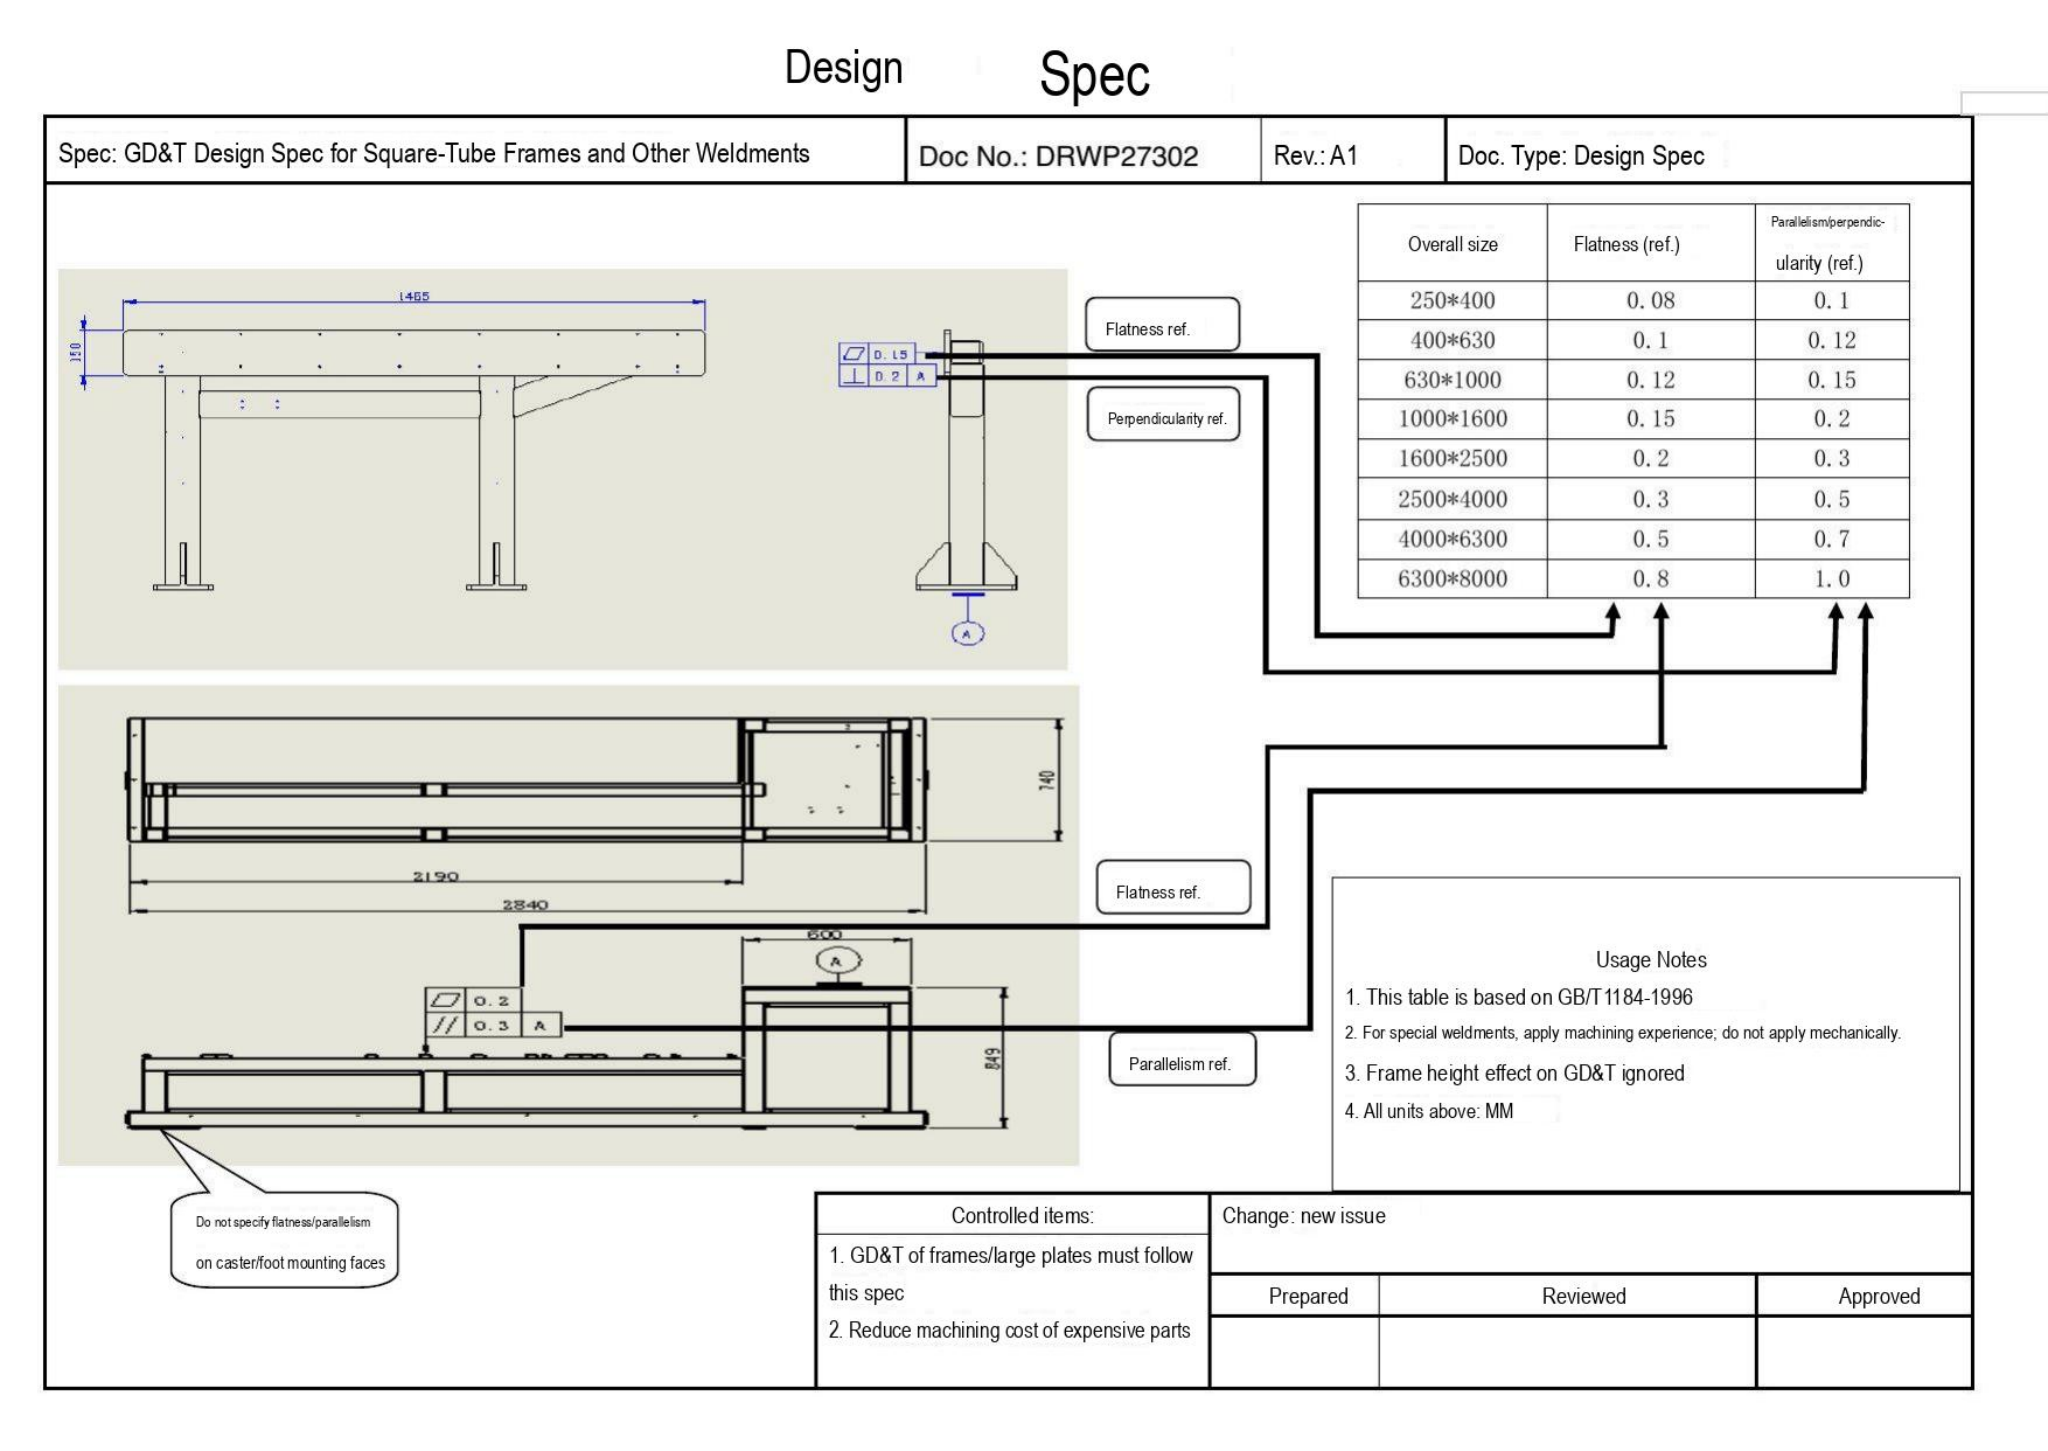Design Spec

| Spec: GD&T Design Spec for Square-Tube Frames and Other Weldments | Doc No.: DRWP27302 | Rev.: A1 | Doc. Type: Design Spec |
|---|---|---|---|

1465

150

0.15

0.2 A

A

Flatness ref.

Perpendicularity ref.

| Overall size | Flatness (ref.) | Parallelism/perpendicularity (ref.) |
|---|---|---|
| 250\*400 | 0.08 | 0.1 |
| 400\*630 | 0.1 | 0.12 |
| 630\*1000 | 0.12 | 0.15 |
| 1000\*1600 | 0.15 | 0.2 |
| 1600\*2500 | 0.2 | 0.3 |
| 2500\*4000 | 0.3 | 0.5 |
| 4000\*6300 | 0.5 | 0.7 |
| 6300\*8000 | 0.8 | 1.0 |

740

2190

2840

Flatness ref.

600

A

0.2

0.3 A

849

Parallelism ref.

Usage Notes
1. This table is based on GB/T1184-1996
2. For special weldments, apply machining experience; do not apply mechanically.
3. Frame height effect on GD&T ignored
4. All units above: MM

Do not specify flatness/parallelism on caster/foot mounting faces

| Controlled items: | Change: new issue | | |
|---|---|---|---|
| 1. GD&T of frames/large plates must follow this spec<br>2. Reduce machining cost of expensive parts | Prepared | Reviewed | Approved |
| | | | |